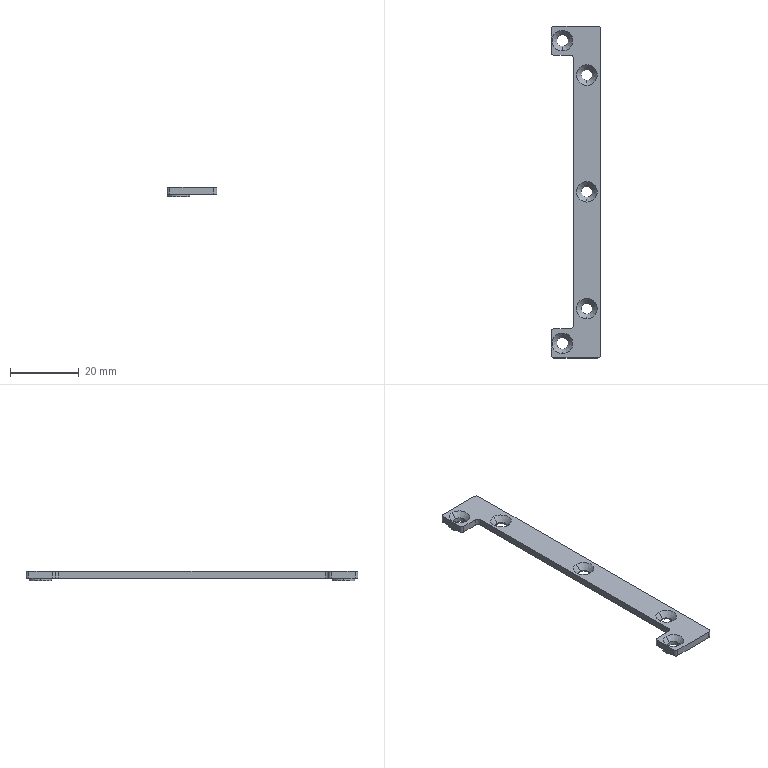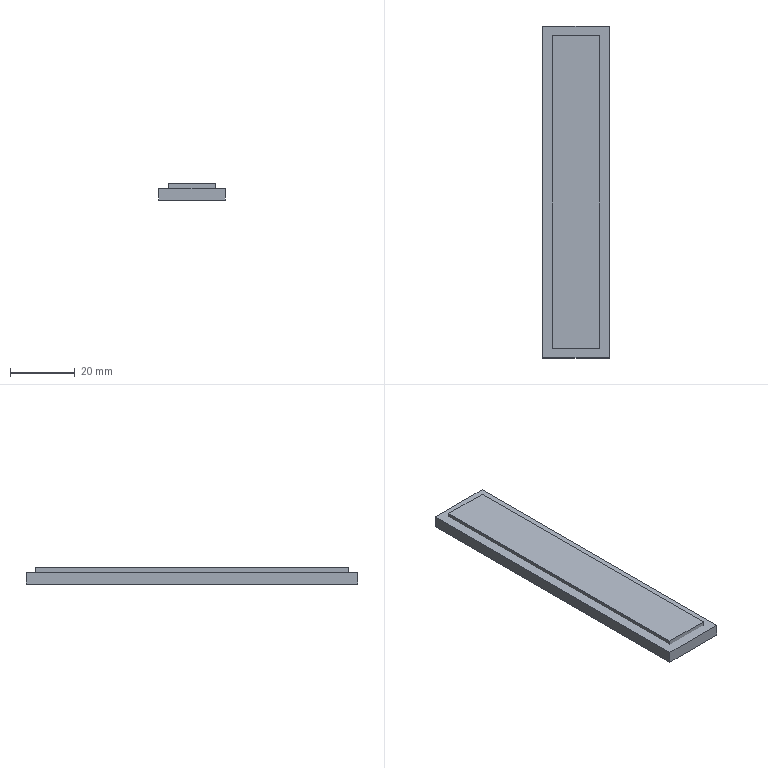CAM job | NX | 3-axis milling, drilling | part box 14.52 x 96.5 x 2.7 mm | stock box 20.52 x 102.5 x 5 mm
Operations:
program,operation,operation_type,tool,method,geometry_group,spindle_rpm,surface_speed,feed_per_tooth,feed_cut,feed_plunge,cut_length_mm,path_length_mm,cut_time_min,machine_time_min
1,FLOOR_WALL,VolumeBased25DMillingOperation,D6,METHOD,A,9500.0,179.0,0.0789,1500.0,100.0,898.117,952.117,0.5987,0.6041
1,DRILLING,Operation,D6A45,METHOD,A,5000.0,94.0,0.025,250.0,0.0,30.0,225.507,0.12,0.1396
1,CAVITY_MILL,CavityMilling,D4,METHOD,A,9500.0,119.0,0.1316,2500.0,1000.0,5628.457,5792.662,2.239,2.255
1,CAVITY_MILL_COPY,CavityMilling,D4,METHOD,A,9500.0,119.0,0.0632,1200.0,1000.0,248.5,311.901,0.2052,0.2115
1,CAVITY_MILL_COPY_1,CavityMilling,D2,METHOD,A,9500.0,59.0,0.0632,1200.0,1000.0,180.653,911.598,0.1056,0.1787
1,HOLE_MILLING,CylinderMilling,D2,METHOD,A,9500.0,59.0,0.0658,1250.0,100.0,312.619,714.04,0.2501,0.2902
1,PLANAR_MILL,PlanarMilling,D6A45,METHOD,A,9500.0,179.0,0.0658,1250.0,100.0,244.248,303.248,0.1954,0.2013
2,FLOOR_WALL_COPY,VolumeBased25DMillingOperation,D6,METHOD,B,9500.0,179.0,0.0789,1500.0,100.0,3245.585,3554.854,2.164,2.195
2,FLOOR_WALL_1,VolumeBased25DMillingOperation,D4,METHOD,B,9500.0,119.0,0.1316,2500.0,1000.0,1332.146,1454.995,0.537,0.5492
2,FLOOR_WALL_1_COPY,VolumeBased25DMillingOperation,D4,METHOD,B,9500.0,119.0,0.0632,1200.0,1000.0,849.539,1498.069,0.7123,0.7771
2,PLANAR_MILL_COPY,PlanarMilling,D6A45,METHOD,B,9500.0,179.0,0.0658,1250.0,100.0,83.209,410.075,0.0666,0.0993
2,PLANAR_MILL_COPY_COPY,PlanarMilling,D6A45,METHOD,B,9500.0,179.0,0.0658,1250.0,100.0,278.22,736.052,0.2226,0.2684